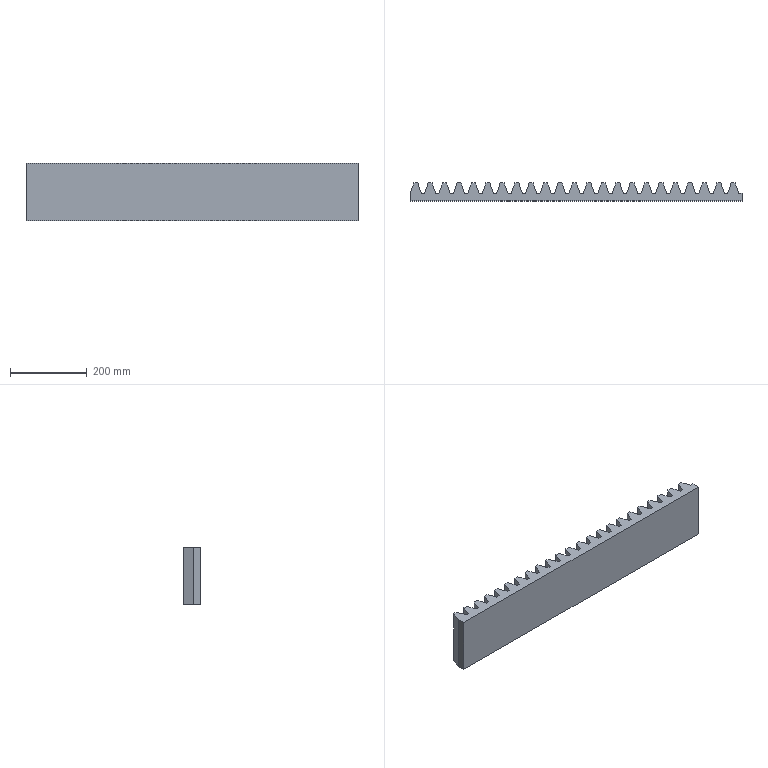Part | SolidWorks | features Extrusion 1, ICE 1 | 1 solid | 97 faces | box 867.08 x 47 x 150 mm | volume 4458786 mm3 | plane 97